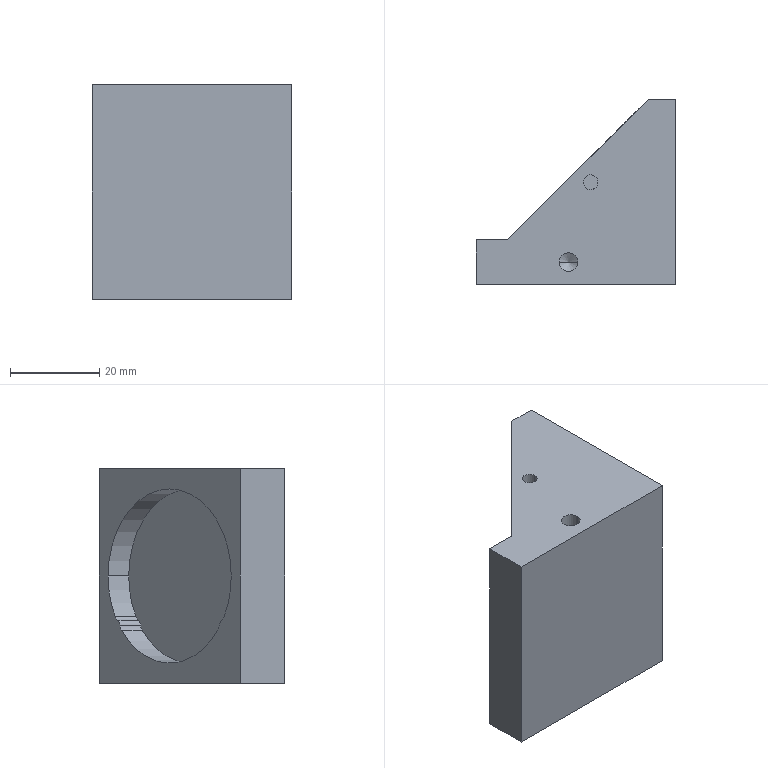Part | SolidWorks | features ICE 7, HoleWzd 3, MoveFace 2, Extrusion 1, Fillet 1, MirrorPattern 1 | 1 solid | 33 faces | box 44.63 x 41.5 x 48 mm | volume 46315 mm3 | cylinder 18 | plane 9 | cone 6 | commonest cylinder face diameters 4.2 x6 5 x4 39 x4 2.895 x2 3.3 x2
STEP:
#1=CARTESIAN_POINT('',(40.23,10.,32.1));
#2=VERTEX_POINT('',#1);
#3=CARTESIAN_POINT('',(40.23,10.,27.9));
#4=VERTEX_POINT('',#3);
#5=CARTESIAN_POINT('',(40.23,10.,30.));
#6=DIRECTION('',(1.,0.,0.));
#7=DIRECTION('',(0.,0.,-1.));
#8=AXIS2_PLACEMENT_3D('',#5,#6,#7);
#9=CIRCLE('',#8,2.1);
#10=EDGE_CURVE('',#2,#4,#9,.T.);
#11=ORIENTED_EDGE('',*,*,#10,.F.);
#12=CARTESIAN_POINT('',(52.63,10.,32.1));
#13=VERTEX_POINT('',#12);
#14=CARTESIAN_POINT('',(54.75,10.,32.1));
#15=DIRECTION('',(1.,0.,0.));
#16=VECTOR('',#15,1000.);
#17=LINE('',#14,#16);
#18=EDGE_CURVE('',#2,#13,#17,.T.);
#19=ORIENTED_EDGE('',*,*,#18,.T.);
#20=CARTESIAN_POINT('',(52.63,10.,27.9));
#21=VERTEX_POINT('',#20);
#22=CARTESIAN_POINT('',(52.63,10.,30.));
#23=DIRECTION('',(1.,0.,0.));
#24=DIRECTION('',(0.,0.,-1.));
#25=AXIS2_PLACEMENT_3D('',#22,#23,#24);
#26=CIRCLE('',#25,2.1);
#27=EDGE_CURVE('',#13,#21,#26,.T.);
#28=ORIENTED_EDGE('',*,*,#27,.T.);
#29=CARTESIAN_POINT('',(54.75,10.,27.9));
#30=DIRECTION('',(1.,0.,0.));
#31=VECTOR('',#30,1000.);
#32=LINE('',#29,#31);
#33=EDGE_CURVE('',#4,#21,#32,.T.);
#34=ORIENTED_EDGE('',*,*,#33,.F.);
#35=EDGE_LOOP('',(#11,#19,#28,#34));
#36=FACE_OUTER_BOUND('',#35,.T.);
#37=CARTESIAN_POINT('',(54.75,10.,30.));
#38=DIRECTION('',(1.,0.,0.));
#39=DIRECTION('',(0.,0.,-1.));
#40=AXIS2_PLACEMENT_3D('',#37,#38,#39);
#41=CYLINDRICAL_SURFACE('',#40,2.1);
#42=ADVANCED_FACE('',(#36),#41,.F.);
#43=CARTESIAN_POINT('',(38.968,10.,30.));
#44=VERTEX_POINT('',#43);
#45=CARTESIAN_POINT('',(40.23,10.,27.9));
#46=DIRECTION('',(0.515,0.,-0.8572));
#47=VECTOR('',#46,1000.);
#48=LINE('',#45,#47);
#49=EDGE_CURVE('',#44,#4,#48,.T.);
#50=ORIENTED_EDGE('',*,*,#49,.F.);
#51=CARTESIAN_POINT('',(40.23,10.,32.1));
#52=DIRECTION('',(0.515,0.,0.8572));
#53=VECTOR('',#52,1000.);
#54=LINE('',#51,#53);
#55=EDGE_CURVE('',#44,#2,#54,.T.);
#56=ORIENTED_EDGE('',*,*,#55,.T.);
#57=ORIENTED_EDGE('',*,*,#10,.T.);
#58=EDGE_LOOP('',(#50,#56,#57));
#59=FACE_OUTER_BOUND('',#58,.T.);
#60=CARTESIAN_POINT('',(40.23,10.,30.));
#61=DIRECTION('',(1.,0.,0.));
#62=DIRECTION('',(0.,0.,-1.));
#63=AXIS2_PLACEMENT_3D('',#60,#61,#62);
#64=CONICAL_SURFACE('',#63,2.1,1.03);
#65=ADVANCED_FACE('',(#59),#64,.F.);
#66=CARTESIAN_POINT('',(26.53,10.,47.6));
#67=VERTEX_POINT('',#66);
#68=CARTESIAN_POINT('',(30.73,10.,47.6));
#69=VERTEX_POINT('',#68);
#70=CARTESIAN_POINT('',(28.63,10.,47.6));
#71=DIRECTION('',(0.,0.,1.));
#72=DIRECTION('',(1.,0.,0.));
#73=AXIS2_PLACEMENT_3D('',#70,#71,#72);
#74=CIRCLE('',#73,2.1);
#75=EDGE_CURVE('',#67,#69,#74,.T.);
#76=ORIENTED_EDGE('',*,*,#75,.F.);
#77=CARTESIAN_POINT('',(26.53,10.,54.));
#78=VERTEX_POINT('',#77);
#79=CARTESIAN_POINT('',(26.53,10.,60.));
#80=DIRECTION('',(0.,0.,1.));
#81=VECTOR('',#80,1000.);
#82=LINE('',#79,#81);
#83=EDGE_CURVE('',#67,#78,#82,.T.);
#84=ORIENTED_EDGE('',*,*,#83,.T.);
#85=CARTESIAN_POINT('',(30.73,10.,54.));
#86=VERTEX_POINT('',#85);
#87=CARTESIAN_POINT('',(28.63,10.,54.));
#88=DIRECTION('',(0.,0.,-1.));
#89=DIRECTION('',(1.,0.,0.));
#90=AXIS2_PLACEMENT_3D('',#87,#88,#89);
#91=CIRCLE('',#90,2.1);
#92=EDGE_CURVE('',#86,#78,#91,.T.);
#93=ORIENTED_EDGE('',*,*,#92,.F.);
#94=CARTESIAN_POINT('',(30.73,10.,60.));
#95=DIRECTION('',(0.,0.,1.));
#96=VECTOR('',#95,1000.);
#97=LINE('',#94,#96);
#98=EDGE_CURVE('',#69,#86,#97,.T.);
#99=ORIENTED_EDGE('',*,*,#98,.F.);
#100=EDGE_LOOP('',(#76,#84,#93,#99));
#101=FACE_OUTER_BOUND('',#100,.T.);
#102=CARTESIAN_POINT('',(28.63,10.,60.));
#103=DIRECTION('',(0.,0.,1.));
#104=DIRECTION('',(1.,0.,0.));
#105=AXIS2_PLACEMENT_3D('',#102,#103,#104);
#106=CYLINDRICAL_SURFACE('',#105,2.1);
#107=ADVANCED_FACE('',(#101),#106,.F.);
#108=CARTESIAN_POINT('',(28.63,10.,46.338));
#109=VERTEX_POINT('',#108);
#110=CARTESIAN_POINT('',(30.73,10.,47.6));
#111=DIRECTION('',(0.8572,0.,0.515));
#112=VECTOR('',#111,1000.);
#113=LINE('',#110,#112);
#114=EDGE_CURVE('',#109,#69,#113,.T.);
#115=ORIENTED_EDGE('',*,*,#114,.F.);
#116=CARTESIAN_POINT('',(26.53,10.,47.6));
#117=DIRECTION('',(-0.8572,0.,0.515));
#118=VECTOR('',#117,1000.);
#119=LINE('',#116,#118);
#120=EDGE_CURVE('',#109,#67,#119,.T.);
#121=ORIENTED_EDGE('',*,*,#120,.T.);
#122=ORIENTED_EDGE('',*,*,#75,.T.);
#123=EDGE_LOOP('',(#115,#121,#122));
#124=FACE_OUTER_BOUND('',#123,.T.);
#125=CARTESIAN_POINT('',(28.63,10.,47.6));
#126=DIRECTION('',(0.,0.,1.));
#127=DIRECTION('',(1.,0.,0.));
#128=AXIS2_PLACEMENT_3D('',#125,#126,#127);
#129=CONICAL_SURFACE('',#128,2.1,1.03);
#130=ADVANCED_FACE('',(#124),#129,.F.);
#131=CARTESIAN_POINT('',(30.73,10.,12.4));
#132=VERTEX_POINT('',#131);
#133=CARTESIAN_POINT('',(26.53,10.,12.4));
#134=VERTEX_POINT('',#133);
#135=CARTESIAN_POINT('',(28.63,10.,12.4));
#136=DIRECTION('',(0.,0.,-1.));
#137=DIRECTION('',(-1.,0.,0.));
#138=AXIS2_PLACEMENT_3D('',#135,#136,#137);
#139=CIRCLE('',#138,2.1);
#140=EDGE_CURVE('',#132,#134,#139,.T.);
#141=ORIENTED_EDGE('',*,*,#140,.F.);
#142=CARTESIAN_POINT('',(30.73,10.,6.));
#143=VERTEX_POINT('',#142);
#144=CARTESIAN_POINT('',(30.73,10.,0.));
#145=DIRECTION('',(0.,0.,-1.));
#146=VECTOR('',#145,1000.);
#147=LINE('',#144,#146);
#148=EDGE_CURVE('',#132,#143,#147,.T.);
#149=ORIENTED_EDGE('',*,*,#148,.T.);
#150=CARTESIAN_POINT('',(26.53,10.,6.));
#151=VERTEX_POINT('',#150);
#152=CARTESIAN_POINT('',(28.63,10.,6.));
#153=DIRECTION('',(0.,0.,1.));
#154=DIRECTION('',(-1.,0.,0.));
#155=AXIS2_PLACEMENT_3D('',#152,#153,#154);
#156=CIRCLE('',#155,2.1);
#157=EDGE_CURVE('',#151,#143,#156,.T.);
#158=ORIENTED_EDGE('',*,*,#157,.F.);
#159=CARTESIAN_POINT('',(26.53,10.,0.));
#160=DIRECTION('',(0.,0.,-1.));
#161=VECTOR('',#160,1000.);
#162=LINE('',#159,#161);
#163=EDGE_CURVE('',#134,#151,#162,.T.);
#164=ORIENTED_EDGE('',*,*,#163,.F.);
#165=EDGE_LOOP('',(#141,#149,#158,#164));
#166=FACE_OUTER_BOUND('',#165,.T.);
#167=CARTESIAN_POINT('',(28.63,10.,0.));
#168=DIRECTION('',(0.,0.,-1.));
#169=DIRECTION('',(-1.,0.,0.));
#170=AXIS2_PLACEMENT_3D('',#167,#168,#169);
#171=CYLINDRICAL_SURFACE('',#170,2.1);
#172=ADVANCED_FACE('',(#166),#171,.F.);
#173=CARTESIAN_POINT('',(28.63,10.,13.662));
#174=VERTEX_POINT('',#173);
#175=CARTESIAN_POINT('',(26.53,10.,12.4));
#176=DIRECTION('',(-0.8572,0.,-0.515));
#177=VECTOR('',#176,1000.);
#178=LINE('',#175,#177);
#179=EDGE_CURVE('',#174,#134,#178,.T.);
#180=ORIENTED_EDGE('',*,*,#179,.F.);
#181=CARTESIAN_POINT('',(30.73,10.,12.4));
#182=DIRECTION('',(0.8572,0.,-0.515));
#183=VECTOR('',#182,1000.);
#184=LINE('',#181,#183);
#185=EDGE_CURVE('',#174,#132,#184,.T.);
#186=ORIENTED_EDGE('',*,*,#185,.T.);
#187=ORIENTED_EDGE('',*,*,#140,.T.);
#188=EDGE_LOOP('',(#180,#186,#187));
#189=FACE_OUTER_BOUND('',#188,.T.);
#190=CARTESIAN_POINT('',(28.63,10.,12.4));
#191=DIRECTION('',(0.,0.,-1.));
#192=DIRECTION('',(-1.,0.,0.));
#193=AXIS2_PLACEMENT_3D('',#190,#191,#192);
#194=CONICAL_SURFACE('',#193,2.1,1.03);
#195=ADVANCED_FACE('',(#189),#194,.F.);
#196=CARTESIAN_POINT('',(49.152,39.925,30.));
#197=VERTEX_POINT('',#196);
#198=CARTESIAN_POINT('',(47.588,38.361,20.979));
#199=VERTEX_POINT('',#198);
#200=CARTESIAN_POINT('',(35.364,26.136,30.));
#201=DIRECTION('',(-0.7071,0.7071,0.));
#202=DIRECTION('',(-0.7071,-0.7071,0.));
#203=AXIS2_PLACEMENT_3D('',#200,#201,#202);
#204=CIRCLE('',#203,19.5);
#205=EDGE_CURVE('',#197,#199,#204,.T.);
#206=ORIENTED_EDGE('',*,*,#205,.F.);
#207=CARTESIAN_POINT('',(44.539,44.539,30.));
#208=VERTEX_POINT('',#207);
#209=CARTESIAN_POINT('',(49.152,39.925,30.));
#210=DIRECTION('',(-0.7071,0.7071,0.));
#211=VECTOR('',#210,1000.);
#212=LINE('',#209,#211);
#213=EDGE_CURVE('',#197,#208,#212,.T.);
#214=ORIENTED_EDGE('',*,*,#213,.T.);
#215=CARTESIAN_POINT('',(42.974,42.974,20.979));
#216=VERTEX_POINT('',#215);
#217=CARTESIAN_POINT('',(30.75,30.75,30.));
#218=DIRECTION('',(-0.7071,0.7071,0.));
#219=DIRECTION('',(-0.7071,-0.7071,0.));
#220=AXIS2_PLACEMENT_3D('',#217,#218,#219);
#221=CIRCLE('',#220,19.5);
#222=EDGE_CURVE('',#208,#216,#221,.T.);
#223=ORIENTED_EDGE('',*,*,#222,.T.);
#224=CARTESIAN_POINT('',(47.588,38.361,20.979));
#225=DIRECTION('',(0.7071,-0.7071,0.));
#226=VECTOR('',#225,1000.);
#227=LINE('',#224,#226);
#228=EDGE_CURVE('',#216,#199,#227,.T.);
#229=ORIENTED_EDGE('',*,*,#228,.T.);
#230=EDGE_LOOP('',(#206,#214,#223,#229));
#231=FACE_OUTER_BOUND('',#230,.T.);
#232=CARTESIAN_POINT('',(35.364,26.136,30.));
#233=DIRECTION('',(-0.7071,0.7071,0.));
#234=DIRECTION('',(-0.7071,-0.7071,0.));
#235=AXIS2_PLACEMENT_3D('',#232,#233,#234);
#236=CYLINDRICAL_SURFACE('',#235,19.5);
#237=ADVANCED_FACE('',(#231),#236,.F.);
#238=ORIENTED_EDGE('',*,*,#213,.F.);
#239=CARTESIAN_POINT('',(21.575,12.348,30.));
#240=VERTEX_POINT('',#239);
#241=CARTESIAN_POINT('',(35.364,26.136,30.));
#242=DIRECTION('',(-0.7071,0.7071,0.));
#243=DIRECTION('',(-0.7071,-0.7071,0.));
#244=AXIS2_PLACEMENT_3D('',#241,#242,#243);
#245=CIRCLE('',#244,19.5);
#246=EDGE_CURVE('',#240,#197,#245,.T.);
#247=ORIENTED_EDGE('',*,*,#246,.F.);
#248=CARTESIAN_POINT('',(16.961,16.961,30.));
#249=VERTEX_POINT('',#248);
#250=CARTESIAN_POINT('',(21.575,12.348,30.));
#251=DIRECTION('',(-0.7071,0.7071,0.));
#252=VECTOR('',#251,1000.);
#253=LINE('',#250,#252);
#254=EDGE_CURVE('',#240,#249,#253,.T.);
#255=ORIENTED_EDGE('',*,*,#254,.T.);
#256=CARTESIAN_POINT('',(30.75,30.75,30.));
#257=DIRECTION('',(-0.7071,0.7071,0.));
#258=DIRECTION('',(-0.7071,-0.7071,0.));
#259=AXIS2_PLACEMENT_3D('',#256,#257,#258);
#260=CIRCLE('',#259,19.5);
#261=EDGE_CURVE('',#249,#208,#260,.T.);
#262=ORIENTED_EDGE('',*,*,#261,.T.);
#263=EDGE_LOOP('',(#238,#247,#255,#262));
#264=FACE_OUTER_BOUND('',#263,.T.);
#265=CARTESIAN_POINT('',(35.228,27.922,49.465));
#266=VERTEX_POINT('',#265);
#267=CARTESIAN_POINT('',(31.928,27.922,49.465));
#268=VERTEX_POINT('',#267);
#269=CARTESIAN_POINT('',(35.228,27.922,49.465));
#270=CARTESIAN_POINT('',(35.228,28.031,49.46));
#271=CARTESIAN_POINT('',(35.218,28.138,49.456));
#272=CARTESIAN_POINT('',(35.176,28.349,49.447));
#273=CARTESIAN_POINT('',(35.144,28.453,49.444));
#274=CARTESIAN_POINT('',(35.061,28.653,49.437));
#275=CARTESIAN_POINT('',(35.011,28.748,49.435));
#276=CARTESIAN_POINT('',(34.891,28.927,49.431));
#277=CARTESIAN_POINT('',(34.821,29.012,49.43));
#278=CARTESIAN_POINT('',(34.593,29.241,49.43));
#279=CARTESIAN_POINT('',(34.408,29.364,49.434));
#280=CARTESIAN_POINT('',(34.011,29.528,49.447));
#281=CARTESIAN_POINT('',(33.794,29.571,49.456));
#282=CARTESIAN_POINT('',(33.471,29.572,49.47));
#283=CARTESIAN_POINT('',(33.362,29.561,49.474));
#284=CARTESIAN_POINT('',(33.151,29.519,49.483));
#285=CARTESIAN_POINT('',(33.048,29.488,49.487));
#286=CARTESIAN_POINT('',(32.848,29.405,49.493));
#287=CARTESIAN_POINT('',(32.751,29.353,49.496));
#288=CARTESIAN_POINT('',(32.572,29.234,49.499));
#289=CARTESIAN_POINT('',(32.489,29.166,49.5));
#290=CARTESIAN_POINT('',(32.335,29.012,49.5));
#291=CARTESIAN_POINT('',(32.267,28.928,49.499));
#292=CARTESIAN_POINT('',(32.147,28.749,49.496));
#293=CARTESIAN_POINT('',(32.095,28.653,49.493));
#294=CARTESIAN_POINT('',(32.013,28.453,49.487));
#295=CARTESIAN_POINT('',(31.981,28.35,49.483));
#296=CARTESIAN_POINT('',(31.939,28.138,49.474));
#297=CARTESIAN_POINT('',(31.928,28.029,49.47));
#298=CARTESIAN_POINT('',(31.928,27.922,49.465));
#299=B_SPLINE_CURVE_WITH_KNOTS('',3,(#269,#270,#271,#272,#273,#274,#275,#276,#277,#278,#279,#280,#281,#282,#283,#284,#285,#286,#287,#288,#289,#290,#291,#292,#293,#294,#295,#296,#297,#298),.UNSPECIFIED.,.F.,.F.,(4,2,2,2,2,2,2,2,2,2,2,2,2,2,4),(0.,0.0003226,0.0006451,0.0009677,0.00129,0.001935,0.002581,0.002903,0.003226,0.003548,0.003871,0.004193,0.004516,0.004838,0.005161),.UNSPECIFIED.);
#300=EDGE_CURVE('',#266,#268,#299,.T.);
#301=ORIENTED_EDGE('',*,*,#300,.T.);
#302=CARTESIAN_POINT('',(31.928,27.922,49.465));
#303=CARTESIAN_POINT('',(31.928,27.706,49.456));
#304=CARTESIAN_POINT('',(31.972,27.489,49.447));
#305=CARTESIAN_POINT('',(32.136,27.092,49.434));
#306=CARTESIAN_POINT('',(32.259,26.908,49.43));
#307=CARTESIAN_POINT('',(32.487,26.68,49.43));
#308=CARTESIAN_POINT('',(32.572,26.61,49.431));
#309=CARTESIAN_POINT('',(32.751,26.49,49.434));
#310=CARTESIAN_POINT('',(32.846,26.439,49.437));
#311=CARTESIAN_POINT('',(33.046,26.356,49.444));
#312=CARTESIAN_POINT('',(33.15,26.324,49.447));
#313=CARTESIAN_POINT('',(33.361,26.282,49.456));
#314=CARTESIAN_POINT('',(33.468,26.272,49.46));
#315=CARTESIAN_POINT('',(33.686,26.271,49.47));
#316=CARTESIAN_POINT('',(33.793,26.282,49.474));
#317=CARTESIAN_POINT('',(34.004,26.324,49.483));
#318=CARTESIAN_POINT('',(34.109,26.355,49.486));
#319=CARTESIAN_POINT('',(34.309,26.438,49.493));
#320=CARTESIAN_POINT('',(34.404,26.489,49.496));
#321=CARTESIAN_POINT('',(34.583,26.608,49.499));
#322=CARTESIAN_POINT('',(34.668,26.678,49.5));
#323=CARTESIAN_POINT('',(34.897,26.906,49.5));
#324=CARTESIAN_POINT('',(35.02,27.09,49.496));
#325=CARTESIAN_POINT('',(35.185,27.487,49.483));
#326=CARTESIAN_POINT('',(35.228,27.704,49.474));
#327=CARTESIAN_POINT('',(35.228,27.922,49.465));
#328=B_SPLINE_CURVE_WITH_KNOTS('',3,(#302,#303,#304,#305,#306,#307,#308,#309,#310,#311,#312,#313,#314,#315,#316,#317,#318,#319,#320,#321,#322,#323,#324,#325,#326,#327),.UNSPECIFIED.,.F.,.F.,(4,2,2,2,2,2,2,2,2,2,2,2,4),(0.005161,0.005806,0.006451,0.006773,0.007096,0.007418,0.007741,0.008063,0.008386,0.008708,0.009031,0.009676,0.01032),.UNSPECIFIED.);
#329=EDGE_CURVE('',#268,#266,#328,.T.);
#330=ORIENTED_EDGE('',*,*,#329,.T.);
#331=EDGE_LOOP('',(#301,#330));
#332=FACE_BOUND('',#331,.T.);
#333=CARTESIAN_POINT('',(35.364,26.136,30.));
#334=DIRECTION('',(-0.7071,0.7071,0.));
#335=DIRECTION('',(-0.7071,-0.7071,0.));
#336=AXIS2_PLACEMENT_3D('',#333,#334,#335);
#337=CYLINDRICAL_SURFACE('',#336,19.5);
#338=ADVANCED_FACE('',(#264,#332),#337,.F.);
#339=ORIENTED_EDGE('',*,*,#329,.F.);
#340=CARTESIAN_POINT('',(31.928,27.922,54.));
#341=VERTEX_POINT('',#340);
#342=CARTESIAN_POINT('',(31.928,27.922,60.));
#343=DIRECTION('',(0.,0.,1.));
#344=VECTOR('',#343,1000.);
#345=LINE('',#342,#344);
#346=EDGE_CURVE('',#268,#341,#345,.T.);
#347=ORIENTED_EDGE('',*,*,#346,.T.);
#348=CARTESIAN_POINT('',(35.228,27.922,54.));
#349=VERTEX_POINT('',#348);
#350=CARTESIAN_POINT('',(33.578,27.922,54.));
#351=DIRECTION('',(0.,0.,-1.));
#352=DIRECTION('',(1.,0.,0.));
#353=AXIS2_PLACEMENT_3D('',#350,#351,#352);
#354=CIRCLE('',#353,1.65);
#355=EDGE_CURVE('',#349,#341,#354,.T.);
#356=ORIENTED_EDGE('',*,*,#355,.F.);
#357=CARTESIAN_POINT('',(35.228,27.922,60.));
#358=DIRECTION('',(0.,0.,1.));
#359=VECTOR('',#358,1000.);
#360=LINE('',#357,#359);
#361=EDGE_CURVE('',#266,#349,#360,.T.);
#362=ORIENTED_EDGE('',*,*,#361,.F.);
#363=EDGE_LOOP('',(#339,#347,#356,#362));
#364=FACE_OUTER_BOUND('',#363,.T.);
#365=CARTESIAN_POINT('',(33.578,27.922,60.));
#366=DIRECTION('',(0.,0.,1.));
#367=DIRECTION('',(1.,0.,0.));
#368=AXIS2_PLACEMENT_3D('',#365,#366,#367);
#369=CYLINDRICAL_SURFACE('',#368,1.65);
#370=ADVANCED_FACE('',(#364),#369,.F.);
#371=ORIENTED_EDGE('',*,*,#157,.T.);
#372=CARTESIAN_POINT('',(28.63,10.,6.));
#373=DIRECTION('',(0.,0.,1.));
#374=DIRECTION('',(-1.,0.,0.));
#375=AXIS2_PLACEMENT_3D('',#372,#373,#374);
#376=CIRCLE('',#375,2.1);
#377=EDGE_CURVE('',#143,#151,#376,.T.);
#378=ORIENTED_EDGE('',*,*,#377,.T.);
#379=EDGE_LOOP('',(#371,#378));
#380=FACE_BOUND('',#379,.T.);
#381=CARTESIAN_POINT('',(46.5,46.5,6.));
#382=VERTEX_POINT('',#381);
#383=CARTESIAN_POINT('',(52.63,46.5,6.));
#384=VERTEX_POINT('',#383);
#385=CARTESIAN_POINT('',(46.5,46.5,6.));
#386=DIRECTION('',(1.,0.,0.));
#387=VECTOR('',#386,1000.);
#388=LINE('',#385,#387);
#389=EDGE_CURVE('',#382,#384,#388,.T.);
#390=ORIENTED_EDGE('',*,*,#389,.T.);
#391=CARTESIAN_POINT('',(52.63,5.,6.));
#392=VERTEX_POINT('',#391);
#393=CARTESIAN_POINT('',(52.63,5.,6.));
#394=DIRECTION('',(0.,1.,0.));
#395=VECTOR('',#394,1000.);
#396=LINE('',#393,#395);
#397=EDGE_CURVE('',#392,#384,#396,.T.);
#398=ORIENTED_EDGE('',*,*,#397,.F.);
#399=CARTESIAN_POINT('',(8.,5.,6.));
#400=VERTEX_POINT('',#399);
#401=CARTESIAN_POINT('',(8.,5.,6.));
#402=DIRECTION('',(1.,0.,0.));
#403=VECTOR('',#402,1000.);
#404=LINE('',#401,#403);
#405=EDGE_CURVE('',#400,#392,#404,.T.);
#406=ORIENTED_EDGE('',*,*,#405,.F.);
#407=CARTESIAN_POINT('',(8.,15.,6.));
#408=VERTEX_POINT('',#407);
#409=CARTESIAN_POINT('',(8.,15.,6.));
#410=DIRECTION('',(0.,-1.,0.));
#411=VECTOR('',#410,1000.);
#412=LINE('',#409,#411);
#413=EDGE_CURVE('',#408,#400,#412,.T.);
#414=ORIENTED_EDGE('',*,*,#413,.F.);
#415=CARTESIAN_POINT('',(15.,15.,6.));
#416=VERTEX_POINT('',#415);
#417=CARTESIAN_POINT('',(0.,15.,6.));
#418=DIRECTION('',(1.,0.,0.));
#419=VECTOR('',#418,1000.);
#420=LINE('',#417,#419);
#421=EDGE_CURVE('',#408,#416,#420,.T.);
#422=ORIENTED_EDGE('',*,*,#421,.T.);
#423=CARTESIAN_POINT('',(15.,15.,6.));
#424=DIRECTION('',(0.7071,0.7071,0.));
#425=VECTOR('',#424,1000.);
#426=LINE('',#423,#425);
#427=EDGE_CURVE('',#416,#382,#426,.T.);
#428=ORIENTED_EDGE('',*,*,#427,.T.);
#429=EDGE_LOOP('',(#390,#398,#406,#414,#422,#428));
#430=FACE_OUTER_BOUND('',#429,.T.);
#431=CARTESIAN_POINT('',(0.,0.,6.));
#432=DIRECTION('',(0.,0.,-1.));
#433=DIRECTION('',(-1.,0.,0.));
#434=AXIS2_PLACEMENT_3D('',#431,#432,#433);
#435=PLANE('',#434);
#436=ADVANCED_FACE('',(#380,#430),#435,.T.);
#437=ORIENTED_EDGE('',*,*,#355,.T.);
#438=CARTESIAN_POINT('',(33.578,27.922,54.));
#439=DIRECTION('',(0.,0.,-1.));
#440=DIRECTION('',(1.,0.,0.));
#441=AXIS2_PLACEMENT_3D('',#438,#439,#440);
#442=CIRCLE('',#441,1.65);
#443=EDGE_CURVE('',#341,#349,#442,.T.);
#444=ORIENTED_EDGE('',*,*,#443,.T.);
#445=EDGE_LOOP('',(#437,#444));
#446=FACE_BOUND('',#445,.T.);
#447=ORIENTED_EDGE('',*,*,#92,.T.);
#448=CARTESIAN_POINT('',(28.63,10.,54.));
#449=DIRECTION('',(0.,0.,-1.));
#450=DIRECTION('',(1.,0.,0.));
#451=AXIS2_PLACEMENT_3D('',#448,#449,#450);
#452=CIRCLE('',#451,2.1);
#453=EDGE_CURVE('',#78,#86,#452,.T.);
#454=ORIENTED_EDGE('',*,*,#453,.T.);
#455=EDGE_LOOP('',(#447,#454));
#456=FACE_BOUND('',#455,.T.);
#457=CARTESIAN_POINT('',(8.,5.,54.));
#458=VERTEX_POINT('',#457);
#459=CARTESIAN_POINT('',(8.,15.,54.));
#460=VERTEX_POINT('',#459);
#461=CARTESIAN_POINT('',(8.,0.,54.));
#462=DIRECTION('',(0.,1.,0.));
#463=VECTOR('',#462,1000.);
#464=LINE('',#461,#463);
#465=EDGE_CURVE('',#458,#460,#464,.T.);
#466=ORIENTED_EDGE('',*,*,#465,.F.);
#467=CARTESIAN_POINT('',(52.63,5.,54.));
#468=VERTEX_POINT('',#467);
#469=CARTESIAN_POINT('',(53.2,5.,54.));
#470=DIRECTION('',(-1.,0.,0.));
#471=VECTOR('',#470,1000.);
#472=LINE('',#469,#471);
#473=EDGE_CURVE('',#468,#458,#472,.T.);
#474=ORIENTED_EDGE('',*,*,#473,.F.);
#475=CARTESIAN_POINT('',(52.63,46.5,54.));
#476=VERTEX_POINT('',#475);
#477=CARTESIAN_POINT('',(52.63,46.5,54.));
#478=DIRECTION('',(0.,-1.,0.));
#479=VECTOR('',#478,1000.);
#480=LINE('',#477,#479);
#481=EDGE_CURVE('',#476,#468,#480,.T.);
#482=ORIENTED_EDGE('',*,*,#481,.F.);
#483=CARTESIAN_POINT('',(46.5,46.5,54.));
#484=VERTEX_POINT('',#483);
#485=CARTESIAN_POINT('',(60.,46.5,54.));
#486=DIRECTION('',(-1.,0.,0.));
#487=VECTOR('',#486,1000.);
#488=LINE('',#485,#487);
#489=EDGE_CURVE('',#476,#484,#488,.T.);
#490=ORIENTED_EDGE('',*,*,#489,.T.);
#491=CARTESIAN_POINT('',(15.,15.,54.));
#492=VERTEX_POINT('',#491);
#493=CARTESIAN_POINT('',(46.5,46.5,54.));
#494=DIRECTION('',(-0.7071,-0.7071,0.));
#495=VECTOR('',#494,1000.);
#496=LINE('',#493,#495);
#497=EDGE_CURVE('',#484,#492,#496,.T.);
#498=ORIENTED_EDGE('',*,*,#497,.T.);
#499=CARTESIAN_POINT('',(15.,15.,54.));
#500=DIRECTION('',(-1.,0.,0.));
#501=VECTOR('',#500,1000.);
#502=LINE('',#499,#501);
#503=EDGE_CURVE('',#492,#460,#502,.T.);
#504=ORIENTED_EDGE('',*,*,#503,.T.);
#505=EDGE_LOOP('',(#466,#474,#482,#490,#498,#504));
#506=FACE_OUTER_BOUND('',#505,.T.);
#507=CARTESIAN_POINT('',(0.,0.,54.));
#508=DIRECTION('',(0.,0.,1.));
#509=DIRECTION('',(1.,0.,0.));
#510=AXIS2_PLACEMENT_3D('',#507,#508,#509);
#511=PLANE('',#510);
#512=ADVANCED_FACE('',(#446,#456,#506),#511,.T.);
#513=ORIENTED_EDGE('',*,*,#413,.T.);
#514=CARTESIAN_POINT('',(8.,5.,54.));
#515=DIRECTION('',(0.,0.,-1.));
#516=VECTOR('',#515,1000.);
#517=LINE('',#514,#516);
#518=EDGE_CURVE('',#458,#400,#517,.T.);
#519=ORIENTED_EDGE('',*,*,#518,.F.);
#520=ORIENTED_EDGE('',*,*,#465,.T.);
#521=CARTESIAN_POINT('',(8.,15.,54.));
#522=DIRECTION('',(0.,0.,-1.));
#523=VECTOR('',#522,1000.);
#524=LINE('',#521,#523);
#525=EDGE_CURVE('',#460,#408,#524,.T.);
#526=ORIENTED_EDGE('',*,*,#525,.T.);
#527=EDGE_LOOP('',(#513,#519,#520,#526));
#528=FACE_OUTER_BOUND('',#527,.T.);
#529=CARTESIAN_POINT('',(8.,0.,0.));
#530=DIRECTION('',(-1.,0.,0.));
#531=DIRECTION('',(0.,0.,1.));
#532=AXIS2_PLACEMENT_3D('',#529,#530,#531);
#533=PLANE('',#532);
#534=ADVANCED_FACE('',(#528),#533,.T.);
#535=ORIENTED_EDGE('',*,*,#489,.F.);
#536=CARTESIAN_POINT('',(52.63,46.5,6.));
#537=DIRECTION('',(0.,0.,1.));
#538=VECTOR('',#537,1000.);
#539=LINE('',#536,#538);
#540=EDGE_CURVE('',#384,#476,#539,.T.);
#541=ORIENTED_EDGE('',*,*,#540,.F.);
#542=ORIENTED_EDGE('',*,*,#389,.F.);
#543=CARTESIAN_POINT('',(46.5,46.5,60.));
#544=DIRECTION('',(0.,0.,-1.));
#545=VECTOR('',#544,1000.);
#546=LINE('',#543,#545);
#547=EDGE_CURVE('',#484,#382,#546,.T.);
#548=ORIENTED_EDGE('',*,*,#547,.F.);
#549=EDGE_LOOP('',(#535,#541,#542,#548));
#550=FACE_OUTER_BOUND('',#549,.T.);
#551=CARTESIAN_POINT('',(46.5,46.5,60.));
#552=DIRECTION('',(0.,-1.,0.));
#553=DIRECTION('',(0.,0.,-1.));
#554=AXIS2_PLACEMENT_3D('',#551,#552,#553);
#555=PLANE('',#554);
#556=ADVANCED_FACE('',(#550),#555,.F.);
#557=ORIENTED_EDGE('',*,*,#525,.F.);
#558=ORIENTED_EDGE('',*,*,#503,.F.);
#559=CARTESIAN_POINT('',(15.,15.,60.));
#560=DIRECTION('',(0.,0.,-1.));
#561=VECTOR('',#560,1000.);
#562=LINE('',#559,#561);
#563=EDGE_CURVE('',#492,#416,#562,.T.);
#564=ORIENTED_EDGE('',*,*,#563,.T.);
#565=ORIENTED_EDGE('',*,*,#421,.F.);
#566=EDGE_LOOP('',(#557,#558,#564,#565));
#567=FACE_OUTER_BOUND('',#566,.T.);
#568=CARTESIAN_POINT('',(0.,15.,60.));
#569=DIRECTION('',(0.,-1.,0.));
#570=DIRECTION('',(1.,0.,0.));
#571=AXIS2_PLACEMENT_3D('',#568,#569,#570);
#572=PLANE('',#571);
#573=ADVANCED_FACE('',(#567),#572,.F.);
#574=CARTESIAN_POINT('',(41.497,41.497,17.782));
#575=VERTEX_POINT('',#574);
#576=CARTESIAN_POINT('',(20.003,20.003,17.782));
#577=VERTEX_POINT('',#576);
#578=CARTESIAN_POINT('',(30.75,30.75,30.));
#579=DIRECTION('',(-0.7071,0.7071,0.));
#580=DIRECTION('',(-0.7071,-0.7071,0.));
#581=AXIS2_PLACEMENT_3D('',#578,#579,#580);
#582=CIRCLE('',#581,19.5);
#583=EDGE_CURVE('',#575,#577,#582,.T.);
#584=ORIENTED_EDGE('',*,*,#583,.F.);
#585=CARTESIAN_POINT('',(41.868,41.868,18.991));
#586=VERTEX_POINT('',#585);
#587=CARTESIAN_POINT('',(40.119,40.119,19.349));
#588=DIRECTION('',(0.7071,-0.7071,0.));
#589=DIRECTION('',(0.7071,0.7071,0.));
#590=AXIS2_PLACEMENT_3D('',#587,#588,#589);
#591=CIRCLE('',#590,2.5);
#592=EDGE_CURVE('',#575,#586,#591,.T.);
#593=ORIENTED_EDGE('',*,*,#592,.T.);
#594=CARTESIAN_POINT('',(42.341,42.341,20.013));
#595=VERTEX_POINT('',#594);
#596=CARTESIAN_POINT('',(42.881,42.881,18.784));
#597=DIRECTION('',(0.7071,-0.7071,0.));
#598=DIRECTION('',(0.7071,0.7071,0.));
#599=AXIS2_PLACEMENT_3D('',#596,#597,#598);
#600=CIRCLE('',#599,1.447);
#601=EDGE_CURVE('',#595,#586,#600,.T.);
#602=ORIENTED_EDGE('',*,*,#601,.F.);
#603=CARTESIAN_POINT('',(41.407,41.407,22.136));
#604=DIRECTION('',(0.7071,-0.7071,0.));
#605=DIRECTION('',(0.7071,0.7071,0.));
#606=AXIS2_PLACEMENT_3D('',#603,#604,#605);
#607=CIRCLE('',#606,2.5);
#608=EDGE_CURVE('',#595,#216,#607,.T.);
#609=ORIENTED_EDGE('',*,*,#608,.T.);
#610=ORIENTED_EDGE('',*,*,#222,.F.);
#611=ORIENTED_EDGE('',*,*,#261,.F.);
#612=CARTESIAN_POINT('',(18.526,18.526,20.979));
#613=VERTEX_POINT('',#612);
#614=CARTESIAN_POINT('',(30.75,30.75,30.));
#615=DIRECTION('',(-0.7071,0.7071,0.));
#616=DIRECTION('',(-0.7071,-0.7071,0.));
#617=AXIS2_PLACEMENT_3D('',#614,#615,#616);
#618=CIRCLE('',#617,19.5);
#619=EDGE_CURVE('',#613,#249,#618,.T.);
#620=ORIENTED_EDGE('',*,*,#619,.F.);
#621=CARTESIAN_POINT('',(19.159,19.159,20.013));
#622=VERTEX_POINT('',#621);
#623=CARTESIAN_POINT('',(20.093,20.093,22.136));
#624=DIRECTION('',(0.7071,-0.7071,0.));
#625=DIRECTION('',(0.7071,0.7071,0.));
#626=AXIS2_PLACEMENT_3D('',#623,#624,#625);
#627=CIRCLE('',#626,2.5);
#628=EDGE_CURVE('',#613,#622,#627,.T.);
#629=ORIENTED_EDGE('',*,*,#628,.T.);
#630=CARTESIAN_POINT('',(19.632,19.632,18.991));
#631=VERTEX_POINT('',#630);
#632=CARTESIAN_POINT('',(18.619,18.619,18.784));
#633=DIRECTION('',(0.7071,-0.7071,0.));
#634=DIRECTION('',(-0.7071,-0.7071,0.));
#635=AXIS2_PLACEMENT_3D('',#632,#633,#634);
#636=CIRCLE('',#635,1.447);
#637=EDGE_CURVE('',#631,#622,#636,.T.);
#638=ORIENTED_EDGE('',*,*,#637,.F.);
#639=CARTESIAN_POINT('',(21.381,21.381,19.349));
#640=DIRECTION('',(0.7071,-0.7071,0.));
#641=DIRECTION('',(0.7071,0.7071,0.));
#642=AXIS2_PLACEMENT_3D('',#639,#640,#641);
#643=CIRCLE('',#642,2.5);
#644=EDGE_CURVE('',#631,#577,#643,.T.);
#645=ORIENTED_EDGE('',*,*,#644,.T.);
#646=EDGE_LOOP('',(#584,#593,#602,#609,#610,#611,#620,#629,#638,#645));
#647=FACE_BOUND('',#646,.T.);
#648=ORIENTED_EDGE('',*,*,#497,.F.);
#649=ORIENTED_EDGE('',*,*,#547,.T.);
#650=ORIENTED_EDGE('',*,*,#427,.F.);
#651=ORIENTED_EDGE('',*,*,#563,.F.);
#652=EDGE_LOOP('',(#648,#649,#650,#651));
#653=FACE_OUTER_BOUND('',#652,.T.);
#654=CARTESIAN_POINT('',(15.,15.,60.));
#655=DIRECTION('',(0.7071,-0.7071,0.));
#656=DIRECTION('',(0.7071,0.7071,0.));
#657=AXIS2_PLACEMENT_3D('',#654,#655,#656);
#658=PLANE('',#657);
#659=ADVANCED_FACE('',(#647,#653),#658,.F.);
#660=ORIENTED_EDGE('',*,*,#346,.F.);
#661=ORIENTED_EDGE('',*,*,#300,.F.);
#662=ORIENTED_EDGE('',*,*,#361,.T.);
#663=ORIENTED_EDGE('',*,*,#443,.F.);
#664=EDGE_LOOP('',(#660,#661,#662,#663));
#665=FACE_OUTER_BOUND('',#664,.T.);
#666=CARTESIAN_POINT('',(33.578,27.922,60.));
#667=DIRECTION('',(0.,0.,1.));
#668=DIRECTION('',(1.,0.,0.));
#669=AXIS2_PLACEMENT_3D('',#666,#667,#668);
#670=CYLINDRICAL_SURFACE('',#669,1.65);
#671=ADVANCED_FACE('',(#665),#670,.F.);
#672=ORIENTED_EDGE('',*,*,#601,.T.);
#673=CARTESIAN_POINT('',(46.482,37.254,18.991));
#674=VERTEX_POINT('',#673);
#675=CARTESIAN_POINT('',(46.482,37.254,18.991));
#676=DIRECTION('',(0.7071,-0.7071,0.));
#677=VECTOR('',#676,1000.);
#678=LINE('',#675,#677);
#679=EDGE_CURVE('',#586,#674,#678,.T.);
#680=ORIENTED_EDGE('',*,*,#679,.T.);
#681=CARTESIAN_POINT('',(46.955,37.727,20.013));
#682=VERTEX_POINT('',#681);
#683=CARTESIAN_POINT('',(47.495,38.267,18.784));
#684=DIRECTION('',(0.7071,-0.7071,0.));
#685=DIRECTION('',(0.7071,0.7071,0.));
#686=AXIS2_PLACEMENT_3D('',#683,#684,#685);
#687=CIRCLE('',#686,1.447);
#688=EDGE_CURVE('',#682,#674,#687,.T.);
#689=ORIENTED_EDGE('',*,*,#688,.F.);
#690=CARTESIAN_POINT('',(46.955,37.727,20.013));
#691=DIRECTION('',(-0.7071,0.7071,0.));
#692=VECTOR('',#691,1000.);
#693=LINE('',#690,#692);
#694=EDGE_CURVE('',#682,#595,#693,.T.);
#695=ORIENTED_EDGE('',*,*,#694,.T.);
#696=EDGE_LOOP('',(#672,#680,#689,#695));
#697=FACE_OUTER_BOUND('',#696,.T.);
#698=CARTESIAN_POINT('',(47.495,38.267,18.784));
#699=DIRECTION('',(-0.7071,0.7071,0.));
#700=DIRECTION('',(-0.7071,-0.7071,0.));
#701=AXIS2_PLACEMENT_3D('',#698,#699,#700);
#702=CYLINDRICAL_SURFACE('',#701,1.447);
#703=ADVANCED_FACE('',(#697),#702,.T.);
#704=ORIENTED_EDGE('',*,*,#254,.F.);
#705=CARTESIAN_POINT('',(23.139,13.912,20.979));
#706=VERTEX_POINT('',#705);
#707=CARTESIAN_POINT('',(35.364,26.136,30.));
#708=DIRECTION('',(-0.7071,0.7071,0.));
#709=DIRECTION('',(-0.7071,-0.7071,0.));
#710=AXIS2_PLACEMENT_3D('',#707,#708,#709);
#711=CIRCLE('',#710,19.5);
#712=EDGE_CURVE('',#706,#240,#711,.T.);
#713=ORIENTED_EDGE('',*,*,#712,.F.);
#714=CARTESIAN_POINT('',(23.139,13.912,20.979));
#715=DIRECTION('',(-0.7071,0.7071,0.));
#716=VECTOR('',#715,1000.);
#717=LINE('',#714,#716);
#718=EDGE_CURVE('',#706,#613,#717,.T.);
#719=ORIENTED_EDGE('',*,*,#718,.T.);
#720=ORIENTED_EDGE('',*,*,#619,.T.);
#721=EDGE_LOOP('',(#704,#713,#719,#720));
#722=FACE_OUTER_BOUND('',#721,.T.);
#723=CARTESIAN_POINT('',(35.364,26.136,30.));
#724=DIRECTION('',(-0.7071,0.7071,0.));
#725=DIRECTION('',(-0.7071,-0.7071,0.));
#726=AXIS2_PLACEMENT_3D('',#723,#724,#725);
#727=CYLINDRICAL_SURFACE('',#726,19.5);
#728=ADVANCED_FACE('',(#722),#727,.F.);
#729=CARTESIAN_POINT('',(24.246,15.018,18.991));
#730=VERTEX_POINT('',#729);
#731=CARTESIAN_POINT('',(23.773,14.545,20.013));
#732=VERTEX_POINT('',#731);
#733=CARTESIAN_POINT('',(23.233,14.005,18.784));
#734=DIRECTION('',(0.7071,-0.7071,0.));
#735=DIRECTION('',(-0.7071,-0.7071,0.));
#736=AXIS2_PLACEMENT_3D('',#733,#734,#735);
#737=CIRCLE('',#736,1.447);
#738=EDGE_CURVE('',#730,#732,#737,.T.);
#739=ORIENTED_EDGE('',*,*,#738,.F.);
#740=CARTESIAN_POINT('',(24.246,15.018,18.991));
#741=DIRECTION('',(-0.7071,0.7071,0.));
#742=VECTOR('',#741,1000.);
#743=LINE('',#740,#742);
#744=EDGE_CURVE('',#730,#631,#743,.T.);
#745=ORIENTED_EDGE('',*,*,#744,.T.);
#746=ORIENTED_EDGE('',*,*,#637,.T.);
#747=CARTESIAN_POINT('',(23.773,14.545,20.013));
#748=DIRECTION('',(0.7071,-0.7071,0.));
#749=VECTOR('',#748,1000.);
#750=LINE('',#747,#749);
#751=EDGE_CURVE('',#622,#732,#750,.T.);
#752=ORIENTED_EDGE('',*,*,#751,.T.);
#753=EDGE_LOOP('',(#739,#745,#746,#752));
#754=FACE_OUTER_BOUND('',#753,.T.);
#755=CARTESIAN_POINT('',(23.233,14.005,18.784));
#756=DIRECTION('',(-0.7071,0.7071,0.));
#757=DIRECTION('',(-0.7071,-0.7071,0.));
#758=AXIS2_PLACEMENT_3D('',#755,#756,#757);
#759=CYLINDRICAL_SURFACE('',#758,1.447);
#760=ADVANCED_FACE('',(#754),#759,.T.);
#761=CARTESIAN_POINT('',(46.11,36.883,17.782));
#762=VERTEX_POINT('',#761);
#763=CARTESIAN_POINT('',(24.617,15.39,17.782));
#764=VERTEX_POINT('',#763);
#765=CARTESIAN_POINT('',(35.364,26.136,30.));
#766=DIRECTION('',(-0.7071,0.7071,0.));
#767=DIRECTION('',(-0.7071,-0.7071,0.));
#768=AXIS2_PLACEMENT_3D('',#765,#766,#767);
#769=CIRCLE('',#768,19.5);
#770=EDGE_CURVE('',#762,#764,#769,.T.);
#771=ORIENTED_EDGE('',*,*,#770,.F.);
#772=CARTESIAN_POINT('',(46.11,36.883,17.782));
#773=DIRECTION('',(-0.7071,0.7071,0.));
#774=VECTOR('',#773,1000.);
#775=LINE('',#772,#774);
#776=EDGE_CURVE('',#762,#575,#775,.T.);
#777=ORIENTED_EDGE('',*,*,#776,.T.);
#778=ORIENTED_EDGE('',*,*,#583,.T.);
#779=CARTESIAN_POINT('',(24.617,15.39,17.782));
#780=DIRECTION('',(0.7071,-0.7071,0.));
#781=VECTOR('',#780,1000.);
#782=LINE('',#779,#781);
#783=EDGE_CURVE('',#577,#764,#782,.T.);
#784=ORIENTED_EDGE('',*,*,#783,.T.);
#785=EDGE_LOOP('',(#771,#777,#778,#784));
#786=FACE_OUTER_BOUND('',#785,.T.);
#787=CARTESIAN_POINT('',(35.364,26.136,30.));
#788=DIRECTION('',(-0.7071,0.7071,0.));
#789=DIRECTION('',(-0.7071,-0.7071,0.));
#790=AXIS2_PLACEMENT_3D('',#787,#788,#789);
#791=CYLINDRICAL_SURFACE('',#790,19.5);
#792=ADVANCED_FACE('',(#786),#791,.F.);
#793=ORIENTED_EDGE('',*,*,#688,.T.);
#794=CARTESIAN_POINT('',(44.733,35.505,19.349));
#795=DIRECTION('',(-0.7071,0.7071,0.));
#796=DIRECTION('',(0.7071,0.7071,0.));
#797=AXIS2_PLACEMENT_3D('',#794,#795,#796);
#798=CIRCLE('',#797,2.5);
#799=EDGE_CURVE('',#674,#762,#798,.T.);
#800=ORIENTED_EDGE('',*,*,#799,.T.);
#801=ORIENTED_EDGE('',*,*,#770,.T.);
#802=CARTESIAN_POINT('',(25.995,16.767,19.349));
#803=DIRECTION('',(-0.7071,0.7071,0.));
#804=DIRECTION('',(0.7071,0.7071,0.));
#805=AXIS2_PLACEMENT_3D('',#802,#803,#804);
#806=CIRCLE('',#805,2.5);
#807=EDGE_CURVE('',#764,#730,#806,.T.);
#808=ORIENTED_EDGE('',*,*,#807,.T.);
#809=ORIENTED_EDGE('',*,*,#738,.T.);
#810=CARTESIAN_POINT('',(24.707,15.479,22.136));
#811=DIRECTION('',(-0.7071,0.7071,0.));
#812=DIRECTION('',(0.7071,0.7071,0.));
#813=AXIS2_PLACEMENT_3D('',#810,#811,#812);
#814=CIRCLE('',#813,2.5);
#815=EDGE_CURVE('',#732,#706,#814,.T.);
#816=ORIENTED_EDGE('',*,*,#815,.T.);
#817=ORIENTED_EDGE('',*,*,#712,.T.);
#818=ORIENTED_EDGE('',*,*,#246,.T.);
#819=ORIENTED_EDGE('',*,*,#205,.T.);
#820=CARTESIAN_POINT('',(46.021,36.793,22.136));
#821=DIRECTION('',(-0.7071,0.7071,0.));
#822=DIRECTION('',(0.7071,0.7071,0.));
#823=AXIS2_PLACEMENT_3D('',#820,#821,#822);
#824=CIRCLE('',#823,2.5);
#825=EDGE_CURVE('',#199,#682,#824,.T.);
#826=ORIENTED_EDGE('',*,*,#825,.T.);
#827=EDGE_LOOP('',(#793,#800,#801,#808,#809,#816,#817,#818,#819,#826));
#828=FACE_OUTER_BOUND('',#827,.T.);
#829=CARTESIAN_POINT('',(41.43,32.202,24.392));
#830=DIRECTION('',(0.7071,-0.7071,0.));
#831=DIRECTION('',(0.7071,0.7071,0.));
#832=AXIS2_PLACEMENT_3D('',#829,#830,#831);
#833=PLANE('',#832);
#834=ADVANCED_FACE('',(#828),#833,.F.);
#835=ORIENTED_EDGE('',*,*,#799,.F.);
#836=ORIENTED_EDGE('',*,*,#679,.F.);
#837=ORIENTED_EDGE('',*,*,#592,.F.);
#838=ORIENTED_EDGE('',*,*,#776,.F.);
#839=EDGE_LOOP('',(#835,#836,#837,#838));
#840=FACE_OUTER_BOUND('',#839,.T.);
#841=CARTESIAN_POINT('',(44.733,35.505,19.349));
#842=DIRECTION('',(-0.7071,0.7071,0.));
#843=DIRECTION('',(-0.7071,-0.7071,0.));
#844=AXIS2_PLACEMENT_3D('',#841,#842,#843);
#845=CYLINDRICAL_SURFACE('',#844,2.5);
#846=ADVANCED_FACE('',(#840),#845,.F.);
#847=ORIENTED_EDGE('',*,*,#825,.F.);
#848=ORIENTED_EDGE('',*,*,#228,.F.);
#849=ORIENTED_EDGE('',*,*,#608,.F.);
#850=ORIENTED_EDGE('',*,*,#694,.F.);
#851=EDGE_LOOP('',(#847,#848,#849,#850));
#852=FACE_OUTER_BOUND('',#851,.T.);
#853=CARTESIAN_POINT('',(46.021,36.793,22.136));
#854=DIRECTION('',(-0.7071,0.7071,0.));
#855=DIRECTION('',(-0.7071,-0.7071,0.));
#856=AXIS2_PLACEMENT_3D('',#853,#854,#855);
#857=CYLINDRICAL_SURFACE('',#856,2.5);
#858=ADVANCED_FACE('',(#852),#857,.F.);
#859=ORIENTED_EDGE('',*,*,#807,.F.);
#860=ORIENTED_EDGE('',*,*,#783,.F.);
#861=ORIENTED_EDGE('',*,*,#644,.F.);
#862=ORIENTED_EDGE('',*,*,#744,.F.);
#863=EDGE_LOOP('',(#859,#860,#861,#862));
#864=FACE_OUTER_BOUND('',#863,.T.);
#865=CARTESIAN_POINT('',(25.995,16.767,19.349));
#866=DIRECTION('',(-0.7071,0.7071,0.));
#867=DIRECTION('',(-0.7071,-0.7071,0.));
#868=AXIS2_PLACEMENT_3D('',#865,#866,#867);
#869=CYLINDRICAL_SURFACE('',#868,2.5);
#870=ADVANCED_FACE('',(#864),#869,.F.);
#871=ORIENTED_EDGE('',*,*,#815,.F.);
#872=ORIENTED_EDGE('',*,*,#751,.F.);
#873=ORIENTED_EDGE('',*,*,#628,.F.);
#874=ORIENTED_EDGE('',*,*,#718,.F.);
#875=EDGE_LOOP('',(#871,#872,#873,#874));
#876=FACE_OUTER_BOUND('',#875,.T.);
#877=CARTESIAN_POINT('',(24.707,15.479,22.136));
#878=DIRECTION('',(-0.7071,0.7071,0.));
#879=DIRECTION('',(-0.7071,-0.7071,0.));
#880=AXIS2_PLACEMENT_3D('',#877,#878,#879);
#881=CYLINDRICAL_SURFACE('',#880,2.5);
#882=ADVANCED_FACE('',(#876),#881,.F.);
#883=ORIENTED_EDGE('',*,*,#185,.F.);
#884=ORIENTED_EDGE('',*,*,#179,.T.);
#885=CARTESIAN_POINT('',(28.63,10.,12.4));
#886=DIRECTION('',(0.,0.,-1.));
#887=DIRECTION('',(-1.,0.,0.));
#888=AXIS2_PLACEMENT_3D('',#885,#886,#887);
#889=CIRCLE('',#888,2.1);
#890=EDGE_CURVE('',#134,#132,#889,.T.);
#891=ORIENTED_EDGE('',*,*,#890,.T.);
#892=EDGE_LOOP('',(#883,#884,#891));
#893=FACE_OUTER_BOUND('',#892,.T.);
#894=CARTESIAN_POINT('',(28.63,10.,12.4));
#895=DIRECTION('',(0.,0.,-1.));
#896=DIRECTION('',(-1.,0.,0.));
#897=AXIS2_PLACEMENT_3D('',#894,#895,#896);
#898=CONICAL_SURFACE('',#897,2.1,1.03);
#899=ADVANCED_FACE('',(#893),#898,.F.);
#900=ORIENTED_EDGE('',*,*,#148,.F.);
#901=ORIENTED_EDGE('',*,*,#890,.F.);
#902=ORIENTED_EDGE('',*,*,#163,.T.);
#903=ORIENTED_EDGE('',*,*,#377,.F.);
#904=EDGE_LOOP('',(#900,#901,#902,#903));
#905=FACE_OUTER_BOUND('',#904,.T.);
#906=CARTESIAN_POINT('',(28.63,10.,0.));
#907=DIRECTION('',(0.,0.,-1.));
#908=DIRECTION('',(-1.,0.,0.));
#909=AXIS2_PLACEMENT_3D('',#906,#907,#908);
#910=CYLINDRICAL_SURFACE('',#909,2.1);
#911=ADVANCED_FACE('',(#905),#910,.F.);
#912=ORIENTED_EDGE('',*,*,#120,.F.);
#913=ORIENTED_EDGE('',*,*,#114,.T.);
#914=CARTESIAN_POINT('',(28.63,10.,47.6));
#915=DIRECTION('',(0.,0.,1.));
#916=DIRECTION('',(1.,0.,0.));
#917=AXIS2_PLACEMENT_3D('',#914,#915,#916);
#918=CIRCLE('',#917,2.1);
#919=EDGE_CURVE('',#69,#67,#918,.T.);
#920=ORIENTED_EDGE('',*,*,#919,.T.);
#921=EDGE_LOOP('',(#912,#913,#920));
#922=FACE_OUTER_BOUND('',#921,.T.);
#923=CARTESIAN_POINT('',(28.63,10.,47.6));
#924=DIRECTION('',(0.,0.,1.));
#925=DIRECTION('',(1.,0.,0.));
#926=AXIS2_PLACEMENT_3D('',#923,#924,#925);
#927=CONICAL_SURFACE('',#926,2.1,1.03);
#928=ADVANCED_FACE('',(#922),#927,.F.);
#929=ORIENTED_EDGE('',*,*,#83,.F.);
#930=ORIENTED_EDGE('',*,*,#919,.F.);
#931=ORIENTED_EDGE('',*,*,#98,.T.);
#932=ORIENTED_EDGE('',*,*,#453,.F.);
#933=EDGE_LOOP('',(#929,#930,#931,#932));
#934=FACE_OUTER_BOUND('',#933,.T.);
#935=CARTESIAN_POINT('',(28.63,10.,60.));
#936=DIRECTION('',(0.,0.,1.));
#937=DIRECTION('',(1.,0.,0.));
#938=AXIS2_PLACEMENT_3D('',#935,#936,#937);
#939=CYLINDRICAL_SURFACE('',#938,2.1);
#940=ADVANCED_FACE('',(#934),#939,.F.);
#941=ORIENTED_EDGE('',*,*,#405,.T.);
#942=CARTESIAN_POINT('',(52.63,5.,54.));
#943=DIRECTION('',(0.,0.,-1.));
#944=VECTOR('',#943,1000.);
#945=LINE('',#942,#944);
#946=EDGE_CURVE('',#468,#392,#945,.T.);
#947=ORIENTED_EDGE('',*,*,#946,.F.);
#948=ORIENTED_EDGE('',*,*,#473,.T.);
#949=ORIENTED_EDGE('',*,*,#518,.T.);
#950=EDGE_LOOP('',(#941,#947,#948,#949));
#951=FACE_OUTER_BOUND('',#950,.T.);
#952=CARTESIAN_POINT('',(0.,5.,0.));
#953=DIRECTION('',(0.,-1.,0.));
#954=DIRECTION('',(1.,0.,0.));
#955=AXIS2_PLACEMENT_3D('',#952,#953,#954);
#956=PLANE('',#955);
#957=ADVANCED_FACE('',(#951),#956,.T.);
#958=CARTESIAN_POINT('',(52.63,10.,30.));
#959=DIRECTION('',(1.,0.,0.));
#960=DIRECTION('',(0.,0.,-1.));
#961=AXIS2_PLACEMENT_3D('',#958,#959,#960);
#962=CIRCLE('',#961,2.1);
#963=EDGE_CURVE('',#21,#13,#962,.T.);
#964=ORIENTED_EDGE('',*,*,#963,.F.);
#965=ORIENTED_EDGE('',*,*,#27,.F.);
#966=EDGE_LOOP('',(#964,#965));
#967=FACE_BOUND('',#966,.T.);
#968=ORIENTED_EDGE('',*,*,#540,.T.);
#969=ORIENTED_EDGE('',*,*,#481,.T.);
#970=ORIENTED_EDGE('',*,*,#946,.T.);
#971=ORIENTED_EDGE('',*,*,#397,.T.);
#972=EDGE_LOOP('',(#968,#969,#970,#971));
#973=FACE_OUTER_BOUND('',#972,.T.);
#974=CARTESIAN_POINT('',(52.63,0.,0.));
#975=DIRECTION('',(1.,0.,0.));
#976=DIRECTION('',(0.,1.,0.));
#977=AXIS2_PLACEMENT_3D('',#974,#975,#976);
#978=PLANE('',#977);
#979=ADVANCED_FACE('',(#967,#973),#978,.T.);
#980=ORIENTED_EDGE('',*,*,#55,.F.);
#981=ORIENTED_EDGE('',*,*,#49,.T.);
#982=CARTESIAN_POINT('',(40.23,10.,30.));
#983=DIRECTION('',(1.,0.,0.));
#984=DIRECTION('',(0.,0.,-1.));
#985=AXIS2_PLACEMENT_3D('',#982,#983,#984);
#986=CIRCLE('',#985,2.1);
#987=EDGE_CURVE('',#4,#2,#986,.T.);
#988=ORIENTED_EDGE('',*,*,#987,.T.);
#989=EDGE_LOOP('',(#980,#981,#988));
#990=FACE_OUTER_BOUND('',#989,.T.);
#991=CARTESIAN_POINT('',(40.23,10.,30.));
#992=DIRECTION('',(1.,0.,0.));
#993=DIRECTION('',(0.,0.,-1.));
#994=AXIS2_PLACEMENT_3D('',#991,#992,#993);
#995=CONICAL_SURFACE('',#994,2.1,1.03);
#996=ADVANCED_FACE('',(#990),#995,.F.);
#997=ORIENTED_EDGE('',*,*,#18,.F.);
#998=ORIENTED_EDGE('',*,*,#987,.F.);
#999=ORIENTED_EDGE('',*,*,#33,.T.);
#1000=ORIENTED_EDGE('',*,*,#963,.T.);
#1001=EDGE_LOOP('',(#997,#998,#999,#1000));
#1002=FACE_OUTER_BOUND('',#1001,.T.);
#1003=CARTESIAN_POINT('',(54.75,10.,30.));
#1004=DIRECTION('',(1.,0.,0.));
#1005=DIRECTION('',(0.,0.,-1.));
#1006=AXIS2_PLACEMENT_3D('',#1003,#1004,#1005);
#1007=CYLINDRICAL_SURFACE('',#1006,2.1);
#1008=ADVANCED_FACE('',(#1002),#1007,.F.);
#1009=CLOSED_SHELL('',(#42,#65,#107,#130,#172,#195,#237,#338,#370,#436,#512,#534,#556,#573,#659,#671,#703,#728,#760,#792,#834,#846,#858,#870,#882,#899,#911,#928,#940,#957,#979,#996,#1008));
#1010=MANIFOLD_SOLID_BREP('',#1009);
#1011=CARTESIAN_POINT('',(0.,0.,0.));
#1012=DIRECTION('',(0.,0.,1.));
#1013=DIRECTION('',(1.,0.,0.));
#1014=AXIS2_PLACEMENT_3D('',#1011,#1012,#1013);
#1015=(LENGTH_UNIT()NAMED_UNIT(*)SI_UNIT(.MILLI.,.METRE.));
#1016=UNCERTAINTY_MEASURE_WITH_UNIT(LENGTH_MEASURE(0.00001),#1015,'','');
#1017=(NAMED_UNIT(*)PLANE_ANGLE_UNIT()SI_UNIT($,.RADIAN.));
#1018=(NAMED_UNIT(*)SI_UNIT($,.STERADIAN.)SOLID_ANGLE_UNIT());
#1019=(GEOMETRIC_REPRESENTATION_CONTEXT(3)GLOBAL_UNCERTAINTY_ASSIGNED_CONTEXT((#1016))GLOBAL_UNIT_ASSIGNED_CONTEXT((#1015,#1017,#1018))REPRESENTATION_CONTEXT('',''));
#1020=ADVANCED_BREP_SHAPE_REPRESENTATION('',(#1010,#1014),#1019);